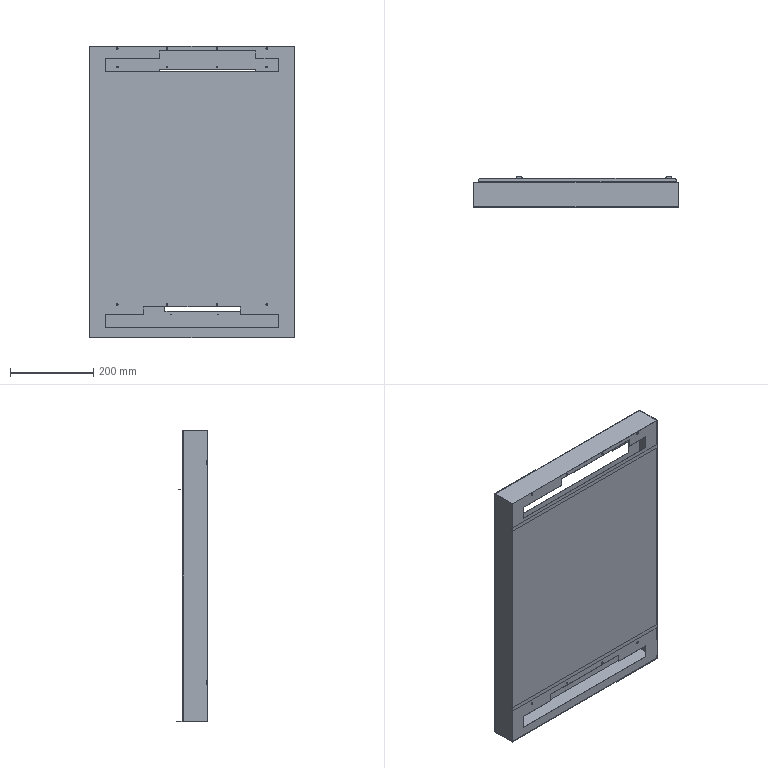Part | STEP file | SOLID | 1 solid | 271 faces | box 493 x 75 x 702 mm | volume 761842 mm3 | cylinder 103 | cone 88 | plane 80 | commonest cylinder face diameters 3.3 x32 2 x24 2.5 x20 7.9 x8 10 x6 5 x4